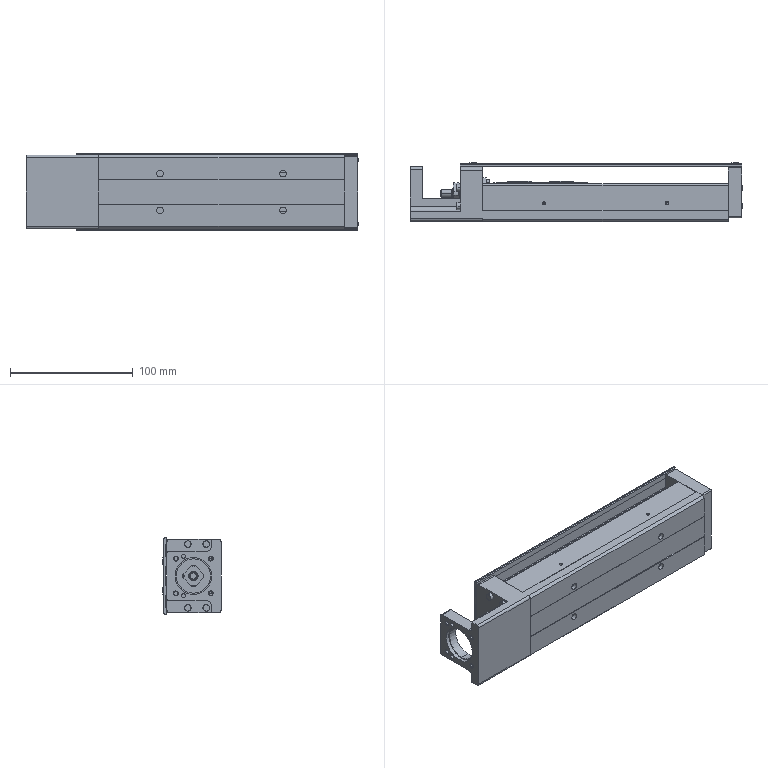Part | STEP file | KR3310A-0100-0-10A0 rail | 3 solids | 572 faces | box 270 x 48.2 x 62 mm | volume 372250 mm3 | plane 271 | cylinder 181 | cone 98 | spline 22 | commonest cylinder face diameters 5.5 x28 2.113 x12 8 x12 4 x10 4.5 x10 1.567 x8